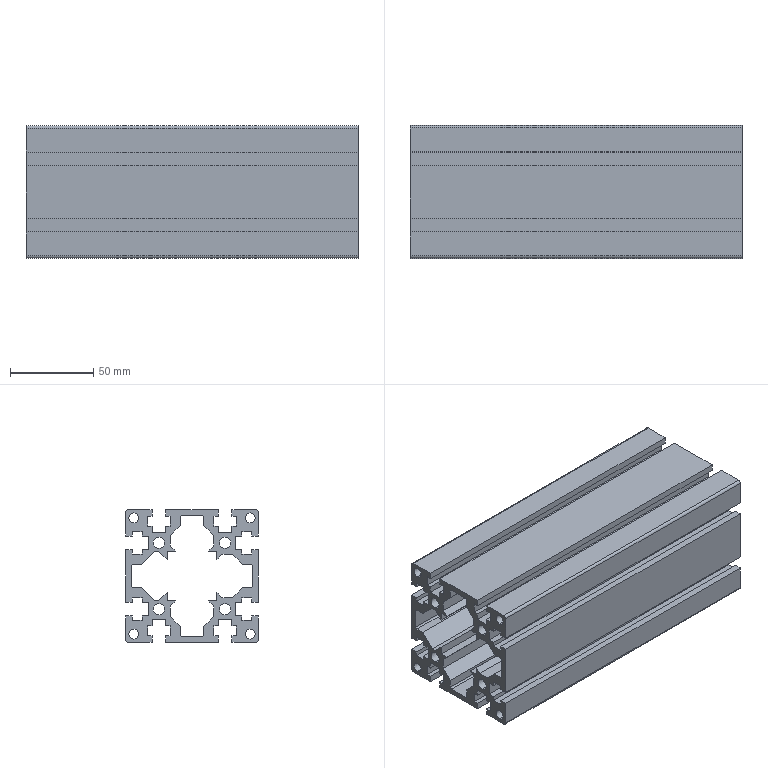Part | SolidWorks | features ICE 1, WeldMemberFeat 1, WeldmentFeature 1 | 1 solid | 174 faces | box 200 x 80 x 80 mm | volume 457804 mm3 | plane 146 | cylinder 28 | commonest cylinder face diameters 2 x8 6 x8 6.8 x8 3 x4